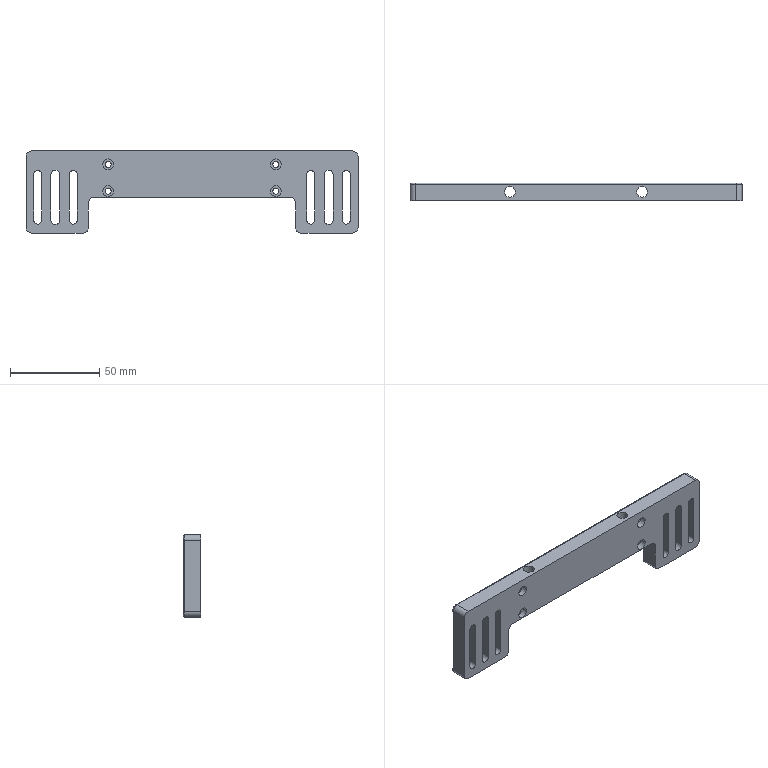CAM job | NX | 3+2 milling, drilling | part box 186 x 10 x 46 mm | stock box 191 x 12 x 50 mm
Tools:
number,name,description,diameter,corner_radius,flute_length,length,flutes
4,D4,平底铣刀-粗,4.0,0.0,25.0,75.0,2
6,D6,平底铣刀-粗,6.0,0.0,25.0,75.0,2
9,D10,平底铣刀-粗,10.0,0.0,35.0,75.0,2
17,D3-J,平底铣刀-精,3.0,0.0,50.0,75.0,2
11,D4-J,平底铣刀-精,4.0,0.0,50.0,75.0,2
7,D6-J,平底铣刀-精,6.0,0.0,25.0,75.0,2
10,D10-J,平底铣刀-精,10.0,0.0,35.0,75.0,2
18,D4R0.5,圆鼻刀-粗,4.0,0.5,50.0,75.0,2
2,D6倒角刀,倒角刀,6.0,0.0,3.0,25.0,2
13,ZT3.4,钻头,3.4,0.0,35.0,50.0,2
Operations:
program,operation,operation_type,tool,method,geometry_group,spindle_rpm,surface_speed,feed_per_tooth,feed_cut,feed_plunge,cut_length_mm,path_length_mm,cut_time_min,machine_time_min
B,动态开粗D10_COPY,CavityMilling,D10,动态开粗-切深K-步距K,W-B,8000.0,251.32,0.25,4000.0,100.0,17264.441,17300.241,4.316,4.32
B,铣沉头_1,CylinderMilling,D4,METHOD,W-B,6000.0,75.398,0.1,1200.0,100.0,467.722,764.122,0.3898,0.4194
B,铣孔_1,CylinderMilling,D4,METHOD,W-B,6000.0,75.398,0.05,600.0,100.0,37.039,348.239,0.0617,0.0929
B,铣倒角_1,PlanarMilling,D6倒角刀,METHOD,W-B,7000.0,131.947,0.0429,600.0,100.0,43.871,340.261,0.0731,0.1028
B,平面去毛刺6X45L_COPY,SurfaceContour,D6倒角刀,爬面_倒角-切深0-步距G,W-B,6500.0,122.519,0.1154,1500.0,100.0,947.383,1415.375,0.6316,0.6784
B,底壁铣飞面精光_COPY_1,VolumeBased25DMillingOperation,D10-J,侧刃精光-切深K-步距G,W-B,8000.0,251.32,0.0625,1000.0,100.0,1436.013,1472.013,1.436,1.44
A,C0.3封闭铣廓倒角6X45L_COPY,PlanarMilling,D6倒角刀,爬面_倒角-切深0-步距G,W-A,7000.0,131.0,0.1071,1500.0,100.0,512.587,548.587,0.3417,0.3453
A,底壁铣飞面精光_COPY,VolumeBased25DMillingOperation,D10-J,侧刃精光-切深K-步距G,W-A,8000.0,251.32,0.0625,1000.0,100.0,1436.013,1472.013,1.436,1.44
A,型腔铣开粗-中_COPY,CavityMilling,D10,分层开粗-切深K-步距G,W-A,8000.0,251.32,0.25,4000.0,100.0,18207.567,19965.018,4.552,4.836
A,打点-深0.8,Operation,D6倒角刀,NONE,W-A,8000.0,150.796,0.0312,500.0,90.0,7.2,185.472,0.0144,0.0322
A,通孔-3-4,Operation,ZT3.4,NONE,W-A,3000.0,32.044,0.0333,200.0,90.0,52.0,275.072,0.26,0.2823
A,底壁粗_1,VolumeBased25DMillingOperation,D6,METHOD,W-A,6000.0,113.0,0.2083,3500.0,100.0,369.499,431.716,0.1056,0.1118
A,底壁粗_2,VolumeBased25DMillingOperation,D6,METHOD,W-A,6000.0,113.0,0.2083,3500.0,100.0,369.499,431.716,0.1056,0.1118
A,通腰槽粗_1,VolumeBased25DMillingOperation,D4,METHOD,W-A,6000.0,75.0,0.1667,2000.0,100.0,7655.427,7905.428,3.828,3.853
A,通腰槽粗_2,VolumeBased25DMillingOperation,D4,METHOD,W-A,6000.0,75.398,0.1667,2000.0,100.0,8940.207,9307.221,4.47,4.507
A,清角D4,ZLevelMilling,D3-J,METHOD,W-A,6000.0,56.549,0.1667,2000.0,80.0,342.336,510.581,0.1714,0.1882
A,腰槽精_1,VolumeBased25DMillingOperation,D4-J,METHOD,W-A,6000.0,113.0,0.0417,500.0,100.0,225.48,518.78,0.451,0.4803
A,腰槽精_2,VolumeBased25DMillingOperation,D4-J,METHOD,W-A,6000.0,113.0,0.0417,500.0,100.0,438.393,895.023,0.8768,0.9224
A,底精_1,VolumeBased25DMillingOperation,D6-J,METHOD,W-A,6000.0,113.0,0.2083,1200.0,100.0,56.5,99.5,0.0471,0.0514
A,底精_2,VolumeBased25DMillingOperation,D6-J,METHOD,W-A,6000.0,113.0,0.2083,1200.0,100.0,56.5,99.5,0.0471,0.0514
A,外形侧面,ZLevelMilling,D3-J,METHOD,W-A,9000.0,84.823,0.1389,2500.0,80.0,804.222,973.74,0.3219,0.3388
A,等高精光往复爬面_COPY,ZLevelMilling,D4R0.5,等高爬面-切深K-步距G,W-A,7000.0,87.965,0.3214,4500.0,100.0,12100.323,12149.868,2.689,2.694
A,仅选体,SurfaceContour,D6倒角刀,METHOD,W-A,8000.0,150.796,0.1875,3000.0,100.0,552.506,1217.986,0.1842,0.2507
A,钻倒角_1,Operation,D6倒角刀,METHOD,W-A,8000.0,150.796,0.0312,500.0,0.0,20.0,217.642,0.04,0.0598
A,底侧精_3,VolumeBased25DMillingOperation,D6-J,METHOD,W-A,6000.0,113.0,0.2083,1200.0,100.0,53.842,96.832,0.0449,0.0492
A,底侧精_4,VolumeBased25DMillingOperation,D6-J,METHOD,W-A,6000.0,113.0,0.2083,1200.0,100.0,53.842,96.832,0.0449,0.0492
A,外形半精_2,VolumeBased25DMillingOperation,D6-J,METHOD,W-A,8000.0,251.327,0.0625,1000.0,100.0,517.519,576.719,0.5175,0.5234